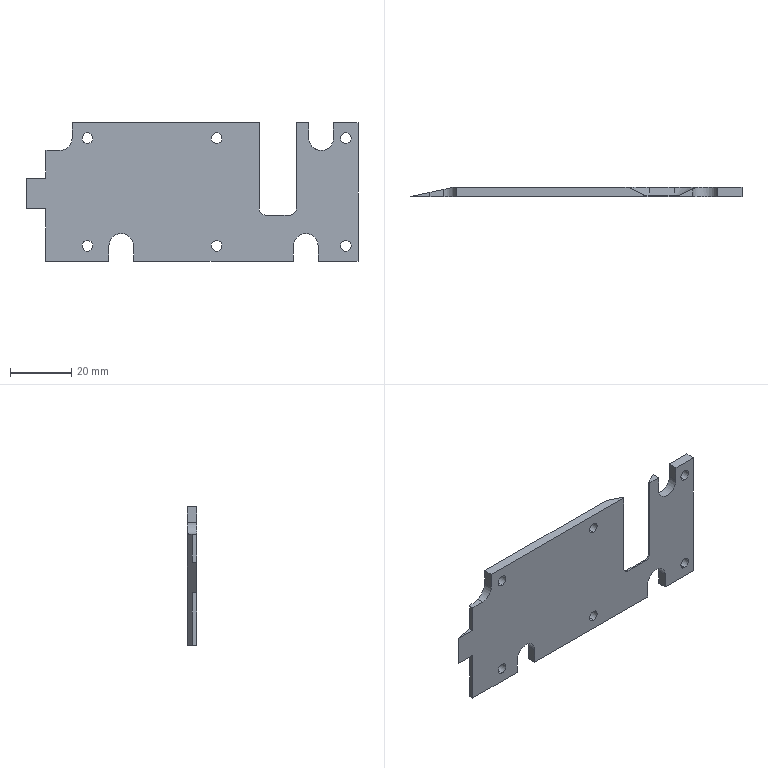Part | SolidWorks | features ICE 6, Chamfer 1, Cut 1, Extrusion 1, Fillet 1 | 1 solid | 50 faces | box 108 x 3 x 45 mm | volume 11001 mm3 | plane 28 | cylinder 20 | cone 2 | commonest cylinder face diameters 3.5 x12 8 x6 4 x2